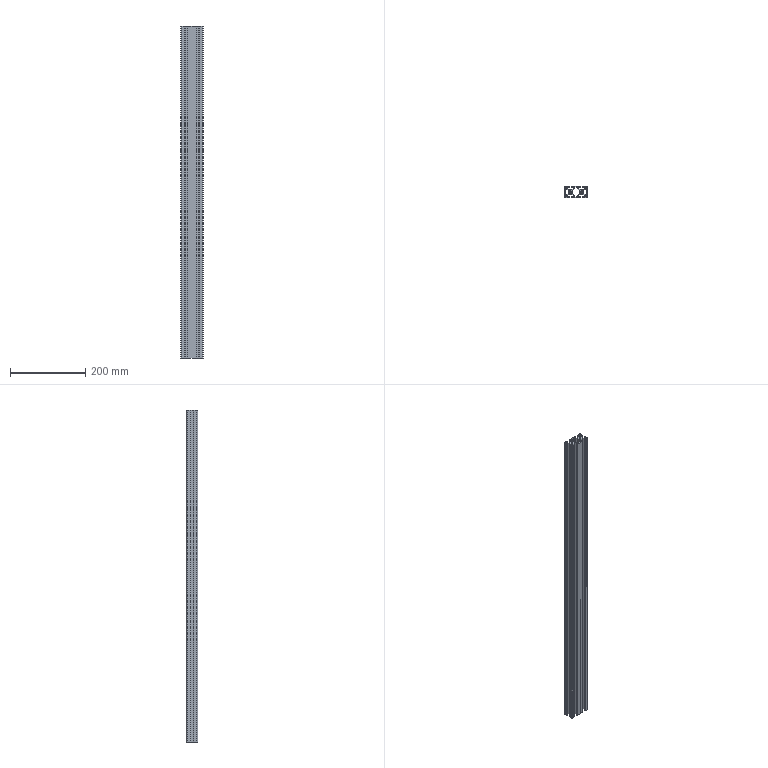Part | STEP file | SynoNew-0304-050 | 1 solid | 236 faces | box 60 x 30 x 880 mm | volume 527129 mm3 | cylinder 118 | plane 118 | commonest cylinder face diameters 0.6 x36 1.6 x36 4 x28 3 x8 6 x4 7 x4